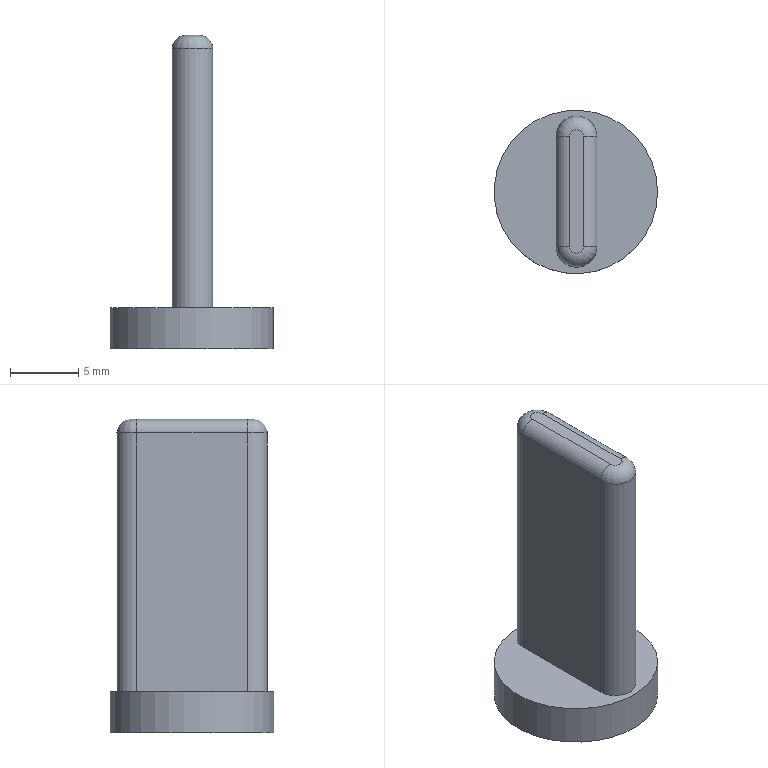Part | NX | features DATUM_CSYS 3, EXTRUDE 2, SKETCH 2, BLEND 1 | 1 solid | 12 faces | box 12 x 12 x 23 mm | volume 960.161 mm3 | plane 5 | cylinder 5 | torus 2 | commonest cylinder face diameters 2 x2 3 x2 12 x1
STEP:
#1=CARTESIAN_POINT('',(6.,0.,3.));
#2=VERTEX_POINT('',#1);
#3=CARTESIAN_POINT('',(0.,0.,3.));
#4=DIRECTION('',(0.,0.,1.));
#5=DIRECTION('',(1.,0.,0.));
#6=AXIS2_PLACEMENT_3D('',#3,#4,#5);
#7=CIRCLE('',#6,6.);
#8=EDGE_CURVE('',#2,#2,#7,.T.);
#9=ORIENTED_EDGE('',*,*,#8,.T.);
#10=EDGE_LOOP('',(#9));
#11=FACE_BOUND('',#10,.T.);
#12=CARTESIAN_POINT('',(-1.451,4.039,3.));
#13=VERTEX_POINT('',#12);
#14=CARTESIAN_POINT('',(-1.451,-4.039,3.));
#15=VERTEX_POINT('',#14);
#16=CARTESIAN_POINT('',(-1.451,4.039,3.));
#17=DIRECTION('',(0.,-1.,0.));
#18=VECTOR('',#17,1000.);
#19=LINE('',#16,#18);
#20=EDGE_CURVE('',#13,#15,#19,.T.);
#21=ORIENTED_EDGE('',*,*,#20,.F.);
#22=CARTESIAN_POINT('',(1.549,4.039,3.));
#23=VERTEX_POINT('',#22);
#24=CARTESIAN_POINT('',(0.04862,4.039,3.));
#25=DIRECTION('',(0.,0.,1.));
#26=DIRECTION('',(1.,0.,0.));
#27=AXIS2_PLACEMENT_3D('',#24,#25,#26);
#28=CIRCLE('',#27,1.5);
#29=EDGE_CURVE('',#23,#13,#28,.T.);
#30=ORIENTED_EDGE('',*,*,#29,.F.);
#31=CARTESIAN_POINT('',(1.549,-4.039,3.));
#32=VERTEX_POINT('',#31);
#33=CARTESIAN_POINT('',(1.549,-4.039,3.));
#34=DIRECTION('',(0.,1.,0.));
#35=VECTOR('',#34,1000.);
#36=LINE('',#33,#35);
#37=EDGE_CURVE('',#32,#23,#36,.T.);
#38=ORIENTED_EDGE('',*,*,#37,.F.);
#39=CARTESIAN_POINT('',(0.04862,-4.039,3.));
#40=DIRECTION('',(0.,0.,1.));
#41=DIRECTION('',(1.,0.,0.));
#42=AXIS2_PLACEMENT_3D('',#39,#40,#41);
#43=CIRCLE('',#42,1.5);
#44=EDGE_CURVE('',#15,#32,#43,.T.);
#45=ORIENTED_EDGE('',*,*,#44,.F.);
#46=EDGE_LOOP('',(#21,#30,#38,#45));
#47=FACE_BOUND('',#46,.T.);
#48=CARTESIAN_POINT('',(0.,0.,3.));
#49=DIRECTION('',(0.,0.,1.));
#50=DIRECTION('',(1.,0.,0.));
#51=AXIS2_PLACEMENT_3D('',#48,#49,#50);
#52=PLANE('',#51);
#53=ADVANCED_FACE('',(#11,#47),#52,.T.);
#54=ORIENTED_EDGE('',*,*,#8,.F.);
#55=EDGE_LOOP('',(#54));
#56=FACE_BOUND('',#55,.T.);
#57=CARTESIAN_POINT('',(6.,0.,0.));
#58=VERTEX_POINT('',#57);
#59=CARTESIAN_POINT('',(0.,0.,0.));
#60=DIRECTION('',(0.,0.,1.));
#61=DIRECTION('',(1.,0.,0.));
#62=AXIS2_PLACEMENT_3D('',#59,#60,#61);
#63=CIRCLE('',#62,6.);
#64=EDGE_CURVE('',#58,#58,#63,.T.);
#65=ORIENTED_EDGE('',*,*,#64,.T.);
#66=EDGE_LOOP('',(#65));
#67=FACE_BOUND('',#66,.T.);
#68=CARTESIAN_POINT('',(0.,0.,3.));
#69=DIRECTION('',(0.,0.,-1.));
#70=DIRECTION('',(-1.,0.,0.));
#71=AXIS2_PLACEMENT_3D('',#68,#69,#70);
#72=CYLINDRICAL_SURFACE('',#71,6.);
#73=ADVANCED_FACE('',(#56,#67),#72,.T.);
#74=ORIENTED_EDGE('',*,*,#64,.F.);
#75=EDGE_LOOP('',(#74));
#76=FACE_BOUND('',#75,.T.);
#77=CARTESIAN_POINT('',(0.,0.,0.));
#78=DIRECTION('',(0.,0.,1.));
#79=DIRECTION('',(1.,0.,0.));
#80=AXIS2_PLACEMENT_3D('',#77,#78,#79);
#81=PLANE('',#80);
#82=ADVANCED_FACE('',(#76),#81,.F.);
#83=CARTESIAN_POINT('',(-1.451,-4.039,22.));
#84=VERTEX_POINT('',#83);
#85=CARTESIAN_POINT('',(-1.451,-4.039,23.));
#86=DIRECTION('',(0.,0.,-1.));
#87=VECTOR('',#86,1000.);
#88=LINE('',#85,#87);
#89=EDGE_CURVE('',#84,#15,#88,.T.);
#90=ORIENTED_EDGE('',*,*,#89,.F.);
#91=CARTESIAN_POINT('',(-1.451,4.039,22.));
#92=VERTEX_POINT('',#91);
#93=CARTESIAN_POINT('',(-1.451,4.039,22.));
#94=DIRECTION('',(0.,-1.,0.));
#95=VECTOR('',#94,1000.);
#96=LINE('',#93,#95);
#97=EDGE_CURVE('',#84,#92,#96,.F.);
#98=ORIENTED_EDGE('',*,*,#97,.T.);
#99=CARTESIAN_POINT('',(-1.451,4.039,23.));
#100=DIRECTION('',(0.,0.,-1.));
#101=VECTOR('',#100,1000.);
#102=LINE('',#99,#101);
#103=EDGE_CURVE('',#92,#13,#102,.T.);
#104=ORIENTED_EDGE('',*,*,#103,.T.);
#105=ORIENTED_EDGE('',*,*,#20,.T.);
#106=EDGE_LOOP('',(#90,#98,#104,#105));
#107=FACE_BOUND('',#106,.T.);
#108=CARTESIAN_POINT('',(-1.451,4.039,23.));
#109=DIRECTION('',(1.,0.,0.));
#110=DIRECTION('',(0.,0.,-1.));
#111=AXIS2_PLACEMENT_3D('',#108,#109,#110);
#112=PLANE('',#111);
#113=ADVANCED_FACE('',(#107),#112,.F.);
#114=CARTESIAN_POINT('',(1.549,-4.039,22.));
#115=VERTEX_POINT('',#114);
#116=CARTESIAN_POINT('',(1.549,-4.039,23.));
#117=DIRECTION('',(0.,0.,-1.));
#118=VECTOR('',#117,1000.);
#119=LINE('',#116,#118);
#120=EDGE_CURVE('',#115,#32,#119,.T.);
#121=ORIENTED_EDGE('',*,*,#120,.F.);
#122=CARTESIAN_POINT('',(0.04862,-4.039,22.));
#123=DIRECTION('',(0.,0.,1.));
#124=DIRECTION('',(1.,0.,0.));
#125=AXIS2_PLACEMENT_3D('',#122,#123,#124);
#126=CIRCLE('',#125,1.5);
#127=EDGE_CURVE('',#115,#84,#126,.F.);
#128=ORIENTED_EDGE('',*,*,#127,.T.);
#129=ORIENTED_EDGE('',*,*,#89,.T.);
#130=ORIENTED_EDGE('',*,*,#44,.T.);
#131=EDGE_LOOP('',(#121,#128,#129,#130));
#132=FACE_BOUND('',#131,.T.);
#133=CARTESIAN_POINT('',(0.04862,-4.039,23.));
#134=DIRECTION('',(0.,0.,-1.));
#135=DIRECTION('',(-1.,0.,0.));
#136=AXIS2_PLACEMENT_3D('',#133,#134,#135);
#137=CYLINDRICAL_SURFACE('',#136,1.5);
#138=ADVANCED_FACE('',(#132),#137,.T.);
#139=CARTESIAN_POINT('',(1.549,4.039,22.));
#140=VERTEX_POINT('',#139);
#141=CARTESIAN_POINT('',(1.549,4.039,23.));
#142=DIRECTION('',(0.,0.,-1.));
#143=VECTOR('',#142,1000.);
#144=LINE('',#141,#143);
#145=EDGE_CURVE('',#140,#23,#144,.T.);
#146=ORIENTED_EDGE('',*,*,#145,.F.);
#147=CARTESIAN_POINT('',(1.549,-4.039,22.));
#148=DIRECTION('',(0.,1.,0.));
#149=VECTOR('',#148,1000.);
#150=LINE('',#147,#149);
#151=EDGE_CURVE('',#140,#115,#150,.F.);
#152=ORIENTED_EDGE('',*,*,#151,.T.);
#153=ORIENTED_EDGE('',*,*,#120,.T.);
#154=ORIENTED_EDGE('',*,*,#37,.T.);
#155=EDGE_LOOP('',(#146,#152,#153,#154));
#156=FACE_BOUND('',#155,.T.);
#157=CARTESIAN_POINT('',(1.549,-4.039,23.));
#158=DIRECTION('',(-1.,0.,0.));
#159=DIRECTION('',(0.,0.,1.));
#160=AXIS2_PLACEMENT_3D('',#157,#158,#159);
#161=PLANE('',#160);
#162=ADVANCED_FACE('',(#156),#161,.F.);
#163=ORIENTED_EDGE('',*,*,#103,.F.);
#164=CARTESIAN_POINT('',(0.04862,4.039,22.));
#165=DIRECTION('',(0.,0.,1.));
#166=DIRECTION('',(1.,0.,0.));
#167=AXIS2_PLACEMENT_3D('',#164,#165,#166);
#168=CIRCLE('',#167,1.5);
#169=EDGE_CURVE('',#92,#140,#168,.F.);
#170=ORIENTED_EDGE('',*,*,#169,.T.);
#171=ORIENTED_EDGE('',*,*,#145,.T.);
#172=ORIENTED_EDGE('',*,*,#29,.T.);
#173=EDGE_LOOP('',(#163,#170,#171,#172));
#174=FACE_BOUND('',#173,.T.);
#175=CARTESIAN_POINT('',(0.04862,4.039,23.));
#176=DIRECTION('',(0.,0.,-1.));
#177=DIRECTION('',(-1.,0.,0.));
#178=AXIS2_PLACEMENT_3D('',#175,#176,#177);
#179=CYLINDRICAL_SURFACE('',#178,1.5);
#180=ADVANCED_FACE('',(#174),#179,.T.);
#181=CARTESIAN_POINT('',(-0.4514,4.039,23.));
#182=VERTEX_POINT('',#181);
#183=CARTESIAN_POINT('',(-0.4514,-4.039,23.));
#184=VERTEX_POINT('',#183);
#185=CARTESIAN_POINT('',(-0.4514,-4.039,23.));
#186=DIRECTION('',(0.,-1.,0.));
#187=VECTOR('',#186,1000.);
#188=LINE('',#185,#187);
#189=EDGE_CURVE('',#182,#184,#188,.T.);
#190=ORIENTED_EDGE('',*,*,#189,.T.);
#191=CARTESIAN_POINT('',(0.5486,-4.039,23.));
#192=VERTEX_POINT('',#191);
#193=CARTESIAN_POINT('',(0.04862,-4.039,23.));
#194=DIRECTION('',(0.,0.,1.));
#195=DIRECTION('',(1.,0.,0.));
#196=AXIS2_PLACEMENT_3D('',#193,#194,#195);
#197=CIRCLE('',#196,0.5);
#198=EDGE_CURVE('',#184,#192,#197,.T.);
#199=ORIENTED_EDGE('',*,*,#198,.T.);
#200=CARTESIAN_POINT('',(0.5486,4.039,23.));
#201=VERTEX_POINT('',#200);
#202=CARTESIAN_POINT('',(0.5486,4.039,23.));
#203=DIRECTION('',(0.,1.,0.));
#204=VECTOR('',#203,1000.);
#205=LINE('',#202,#204);
#206=EDGE_CURVE('',#192,#201,#205,.T.);
#207=ORIENTED_EDGE('',*,*,#206,.T.);
#208=CARTESIAN_POINT('',(0.04862,4.039,23.));
#209=DIRECTION('',(0.,0.,1.));
#210=DIRECTION('',(1.,0.,0.));
#211=AXIS2_PLACEMENT_3D('',#208,#209,#210);
#212=CIRCLE('',#211,0.5);
#213=EDGE_CURVE('',#201,#182,#212,.T.);
#214=ORIENTED_EDGE('',*,*,#213,.T.);
#215=EDGE_LOOP('',(#190,#199,#207,#214));
#216=FACE_BOUND('',#215,.T.);
#217=CARTESIAN_POINT('',(0.04862,-4.039,23.));
#218=DIRECTION('',(0.,0.,1.));
#219=DIRECTION('',(1.,0.,0.));
#220=AXIS2_PLACEMENT_3D('',#217,#218,#219);
#221=PLANE('',#220);
#222=ADVANCED_FACE('',(#216),#221,.T.);
#223=CARTESIAN_POINT('',(0.5486,4.039,22.));
#224=DIRECTION('',(0.,-1.,0.));
#225=DIRECTION('',(0.,0.,-1.));
#226=AXIS2_PLACEMENT_3D('',#223,#224,#225);
#227=CIRCLE('',#226,1.);
#228=EDGE_CURVE('',#140,#201,#227,.T.);
#229=ORIENTED_EDGE('',*,*,#228,.F.);
#230=ORIENTED_EDGE('',*,*,#169,.F.);
#231=CARTESIAN_POINT('',(-0.4514,4.039,22.));
#232=DIRECTION('',(0.,-1.,0.));
#233=DIRECTION('',(0.,0.,-1.));
#234=AXIS2_PLACEMENT_3D('',#231,#232,#233);
#235=CIRCLE('',#234,1.);
#236=EDGE_CURVE('',#182,#92,#235,.T.);
#237=ORIENTED_EDGE('',*,*,#236,.F.);
#238=ORIENTED_EDGE('',*,*,#213,.F.);
#239=EDGE_LOOP('',(#229,#230,#237,#238));
#240=FACE_BOUND('',#239,.T.);
#241=CARTESIAN_POINT('',(0.04862,4.039,22.));
#242=DIRECTION('',(0.,0.,1.));
#243=DIRECTION('',(1.,0.,0.));
#244=AXIS2_PLACEMENT_3D('',#241,#242,#243);
#245=DEGENERATE_TOROIDAL_SURFACE('',#244,0.5,1.,.T.);
#246=ADVANCED_FACE('',(#240),#245,.T.);
#247=ORIENTED_EDGE('',*,*,#236,.T.);
#248=ORIENTED_EDGE('',*,*,#97,.F.);
#249=CARTESIAN_POINT('',(-0.4514,-4.039,22.));
#250=DIRECTION('',(0.,-1.,0.));
#251=DIRECTION('',(1.,0.,0.));
#252=AXIS2_PLACEMENT_3D('',#249,#250,#251);
#253=CIRCLE('',#252,1.);
#254=EDGE_CURVE('',#184,#84,#253,.T.);
#255=ORIENTED_EDGE('',*,*,#254,.F.);
#256=ORIENTED_EDGE('',*,*,#189,.F.);
#257=EDGE_LOOP('',(#247,#248,#255,#256));
#258=FACE_BOUND('',#257,.T.);
#259=CARTESIAN_POINT('',(-0.4514,-4.039,22.));
#260=DIRECTION('',(0.,1.,0.));
#261=DIRECTION('',(0.,0.,1.));
#262=AXIS2_PLACEMENT_3D('',#259,#260,#261);
#263=CYLINDRICAL_SURFACE('',#262,1.);
#264=ADVANCED_FACE('',(#258),#263,.T.);
#265=ORIENTED_EDGE('',*,*,#228,.T.);
#266=ORIENTED_EDGE('',*,*,#206,.F.);
#267=CARTESIAN_POINT('',(0.5486,-4.039,22.));
#268=DIRECTION('',(0.,-1.,0.));
#269=DIRECTION('',(0.,0.,-1.));
#270=AXIS2_PLACEMENT_3D('',#267,#268,#269);
#271=CIRCLE('',#270,1.);
#272=EDGE_CURVE('',#115,#192,#271,.T.);
#273=ORIENTED_EDGE('',*,*,#272,.F.);
#274=ORIENTED_EDGE('',*,*,#151,.F.);
#275=EDGE_LOOP('',(#265,#266,#273,#274));
#276=FACE_BOUND('',#275,.T.);
#277=CARTESIAN_POINT('',(0.5486,-4.039,22.));
#278=DIRECTION('',(0.,-1.,0.));
#279=DIRECTION('',(0.,0.,-1.));
#280=AXIS2_PLACEMENT_3D('',#277,#278,#279);
#281=CYLINDRICAL_SURFACE('',#280,1.);
#282=ADVANCED_FACE('',(#276),#281,.T.);
#283=ORIENTED_EDGE('',*,*,#254,.T.);
#284=ORIENTED_EDGE('',*,*,#127,.F.);
#285=ORIENTED_EDGE('',*,*,#272,.T.);
#286=ORIENTED_EDGE('',*,*,#198,.F.);
#287=EDGE_LOOP('',(#283,#284,#285,#286));
#288=FACE_BOUND('',#287,.T.);
#289=CARTESIAN_POINT('',(0.04862,-4.039,22.));
#290=DIRECTION('',(0.,0.,1.));
#291=DIRECTION('',(1.,0.,0.));
#292=AXIS2_PLACEMENT_3D('',#289,#290,#291);
#293=DEGENERATE_TOROIDAL_SURFACE('',#292,0.5,1.,.T.);
#294=ADVANCED_FACE('',(#288),#293,.T.);
#295=CLOSED_SHELL('',(#53,#73,#82,#113,#138,#162,#180,#222,#246,#264,#282,#294));
#296=MANIFOLD_SOLID_BREP('',#295);
#297=(LENGTH_UNIT()NAMED_UNIT(*)SI_UNIT(.MILLI.,.METRE.));
#298=UNCERTAINTY_MEASURE_WITH_UNIT(LENGTH_MEASURE(0.00001),#297,'','');
#299=(NAMED_UNIT(*)PLANE_ANGLE_UNIT()SI_UNIT($,.RADIAN.));
#300=(NAMED_UNIT(*)SI_UNIT($,.STERADIAN.)SOLID_ANGLE_UNIT());
#301=(GEOMETRIC_REPRESENTATION_CONTEXT(3)GLOBAL_UNCERTAINTY_ASSIGNED_CONTEXT((#298))GLOBAL_UNIT_ASSIGNED_CONTEXT((#297,#299,#300))REPRESENTATION_CONTEXT('',''));
#302=ADVANCED_BREP_SHAPE_REPRESENTATION('',(#296),#301);